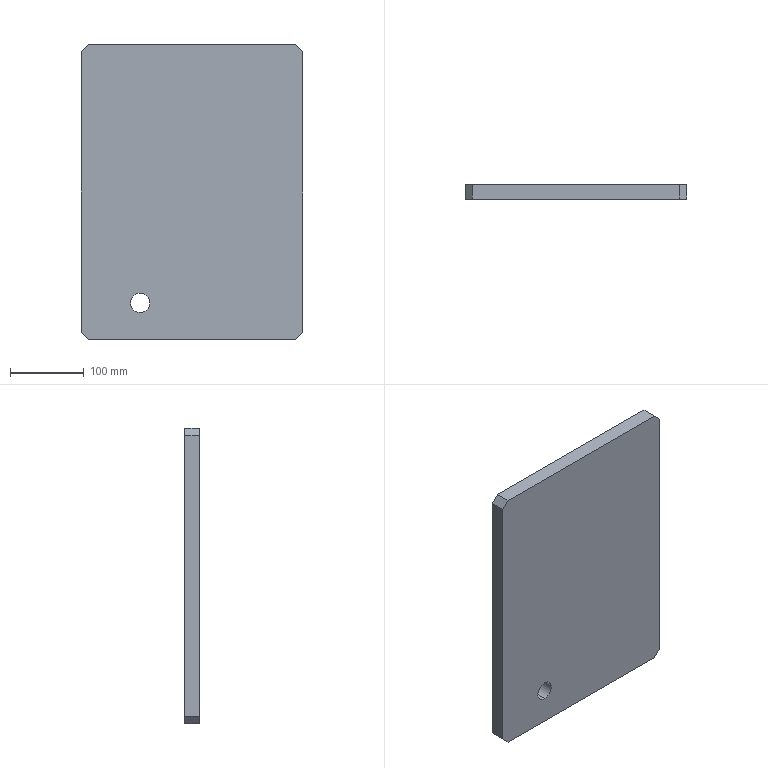Part | SolidWorks | features Chamfer 1, Extrusion 1, HoleWzd 1 | 1 solid | 12 faces | box 300 x 20 x 400 mm | volume 2385381 mm3 | plane 10 | cylinder 2 | commonest cylinder face diameters 26 x2
STEP:
#1=CARTESIAN_POINT('',(-70.,20.,-137.));
#2=VERTEX_POINT('',#1);
#3=CARTESIAN_POINT('',(-70.,20.,-163.));
#4=VERTEX_POINT('',#3);
#5=CARTESIAN_POINT('',(-70.,20.,-150.));
#6=DIRECTION('',(0.,-1.,0.));
#7=DIRECTION('',(0.,0.,-1.));
#8=AXIS2_PLACEMENT_3D('',#5,#6,#7);
#9=CIRCLE('',#8,13.);
#10=EDGE_CURVE('',#2,#4,#9,.T.);
#11=ORIENTED_EDGE('',*,*,#10,.F.);
#12=CARTESIAN_POINT('',(-70.,0.,-137.));
#13=VERTEX_POINT('',#12);
#14=CARTESIAN_POINT('',(-70.,0.,-137.));
#15=DIRECTION('',(0.,-1.,0.));
#16=VECTOR('',#15,1000.);
#17=LINE('',#14,#16);
#18=EDGE_CURVE('',#2,#13,#17,.T.);
#19=ORIENTED_EDGE('',*,*,#18,.T.);
#20=CARTESIAN_POINT('',(-70.,0.,-163.));
#21=VERTEX_POINT('',#20);
#22=CARTESIAN_POINT('',(-70.,0.,-150.));
#23=DIRECTION('',(0.,-1.,0.));
#24=DIRECTION('',(0.,0.,-1.));
#25=AXIS2_PLACEMENT_3D('',#22,#23,#24);
#26=CIRCLE('',#25,13.);
#27=EDGE_CURVE('',#13,#21,#26,.T.);
#28=ORIENTED_EDGE('',*,*,#27,.T.);
#29=CARTESIAN_POINT('',(-70.,0.,-163.));
#30=DIRECTION('',(0.,-1.,0.));
#31=VECTOR('',#30,1000.);
#32=LINE('',#29,#31);
#33=EDGE_CURVE('',#4,#21,#32,.T.);
#34=ORIENTED_EDGE('',*,*,#33,.F.);
#35=EDGE_LOOP('',(#11,#19,#28,#34));
#36=FACE_OUTER_BOUND('',#35,.T.);
#37=CARTESIAN_POINT('',(-70.,0.,-150.));
#38=DIRECTION('',(0.,-1.,0.));
#39=DIRECTION('',(0.,0.,-1.));
#40=AXIS2_PLACEMENT_3D('',#37,#38,#39);
#41=CYLINDRICAL_SURFACE('',#40,13.);
#42=ADVANCED_FACE('',(#36),#41,.F.);
#43=CARTESIAN_POINT('',(150.,20.,190.));
#44=VERTEX_POINT('',#43);
#45=CARTESIAN_POINT('',(150.,20.,-190.));
#46=VERTEX_POINT('',#45);
#47=CARTESIAN_POINT('',(150.,20.,200.));
#48=DIRECTION('',(0.,0.,-1.));
#49=VECTOR('',#48,1000.);
#50=LINE('',#47,#49);
#51=EDGE_CURVE('',#44,#46,#50,.T.);
#52=ORIENTED_EDGE('',*,*,#51,.F.);
#53=CARTESIAN_POINT('',(150.,0.,190.));
#54=VERTEX_POINT('',#53);
#55=CARTESIAN_POINT('',(150.,20.,190.));
#56=DIRECTION('',(0.,-1.,0.));
#57=VECTOR('',#56,1000.);
#58=LINE('',#55,#57);
#59=EDGE_CURVE('',#44,#54,#58,.T.);
#60=ORIENTED_EDGE('',*,*,#59,.T.);
#61=CARTESIAN_POINT('',(150.,0.,-190.));
#62=VERTEX_POINT('',#61);
#63=CARTESIAN_POINT('',(150.,0.,200.));
#64=DIRECTION('',(0.,0.,-1.));
#65=VECTOR('',#64,1000.);
#66=LINE('',#63,#65);
#67=EDGE_CURVE('',#54,#62,#66,.T.);
#68=ORIENTED_EDGE('',*,*,#67,.T.);
#69=CARTESIAN_POINT('',(150.,20.,-190.));
#70=DIRECTION('',(0.,1.,0.));
#71=VECTOR('',#70,1000.);
#72=LINE('',#69,#71);
#73=EDGE_CURVE('',#62,#46,#72,.T.);
#74=ORIENTED_EDGE('',*,*,#73,.T.);
#75=EDGE_LOOP('',(#52,#60,#68,#74));
#76=FACE_OUTER_BOUND('',#75,.T.);
#77=CARTESIAN_POINT('',(150.,20.,200.));
#78=DIRECTION('',(-1.,0.,0.));
#79=DIRECTION('',(0.,0.,1.));
#80=AXIS2_PLACEMENT_3D('',#77,#78,#79);
#81=PLANE('',#80);
#82=ADVANCED_FACE('',(#76),#81,.F.);
#83=CARTESIAN_POINT('',(140.,0.,-200.));
#84=VERTEX_POINT('',#83);
#85=CARTESIAN_POINT('',(-140.,0.,-200.));
#86=VERTEX_POINT('',#85);
#87=CARTESIAN_POINT('',(-150.,0.,-200.));
#88=DIRECTION('',(-1.,0.,0.));
#89=VECTOR('',#88,1000.);
#90=LINE('',#87,#89);
#91=EDGE_CURVE('',#84,#86,#90,.T.);
#92=ORIENTED_EDGE('',*,*,#91,.T.);
#93=CARTESIAN_POINT('',(-140.,20.,-200.));
#94=VERTEX_POINT('',#93);
#95=CARTESIAN_POINT('',(-140.,20.,-200.));
#96=DIRECTION('',(0.,1.,0.));
#97=VECTOR('',#96,1000.);
#98=LINE('',#95,#97);
#99=EDGE_CURVE('',#86,#94,#98,.T.);
#100=ORIENTED_EDGE('',*,*,#99,.T.);
#101=CARTESIAN_POINT('',(140.,20.,-200.));
#102=VERTEX_POINT('',#101);
#103=CARTESIAN_POINT('',(-150.,20.,-200.));
#104=DIRECTION('',(-1.,0.,0.));
#105=VECTOR('',#104,1000.);
#106=LINE('',#103,#105);
#107=EDGE_CURVE('',#102,#94,#106,.T.);
#108=ORIENTED_EDGE('',*,*,#107,.F.);
#109=CARTESIAN_POINT('',(140.,20.,-200.));
#110=DIRECTION('',(0.,-1.,0.));
#111=VECTOR('',#110,1000.);
#112=LINE('',#109,#111);
#113=EDGE_CURVE('',#102,#84,#112,.T.);
#114=ORIENTED_EDGE('',*,*,#113,.T.);
#115=EDGE_LOOP('',(#92,#100,#108,#114));
#116=FACE_OUTER_BOUND('',#115,.T.);
#117=CARTESIAN_POINT('',(-150.,20.,-200.));
#118=DIRECTION('',(0.,0.,1.));
#119=DIRECTION('',(1.,0.,0.));
#120=AXIS2_PLACEMENT_3D('',#117,#118,#119);
#121=PLANE('',#120);
#122=ADVANCED_FACE('',(#116),#121,.F.);
#123=CARTESIAN_POINT('',(-150.,0.,-190.));
#124=VERTEX_POINT('',#123);
#125=CARTESIAN_POINT('',(-150.,0.,190.));
#126=VERTEX_POINT('',#125);
#127=CARTESIAN_POINT('',(-150.,0.,200.));
#128=DIRECTION('',(0.,0.,1.));
#129=VECTOR('',#128,1000.);
#130=LINE('',#127,#129);
#131=EDGE_CURVE('',#124,#126,#130,.T.);
#132=ORIENTED_EDGE('',*,*,#131,.T.);
#133=CARTESIAN_POINT('',(-150.,20.,190.));
#134=VERTEX_POINT('',#133);
#135=CARTESIAN_POINT('',(-150.,20.,190.));
#136=DIRECTION('',(0.,1.,0.));
#137=VECTOR('',#136,1000.);
#138=LINE('',#135,#137);
#139=EDGE_CURVE('',#126,#134,#138,.T.);
#140=ORIENTED_EDGE('',*,*,#139,.T.);
#141=CARTESIAN_POINT('',(-150.,20.,-190.));
#142=VERTEX_POINT('',#141);
#143=CARTESIAN_POINT('',(-150.,20.,200.));
#144=DIRECTION('',(0.,0.,1.));
#145=VECTOR('',#144,1000.);
#146=LINE('',#143,#145);
#147=EDGE_CURVE('',#142,#134,#146,.T.);
#148=ORIENTED_EDGE('',*,*,#147,.F.);
#149=CARTESIAN_POINT('',(-150.,20.,-190.));
#150=DIRECTION('',(0.,-1.,0.));
#151=VECTOR('',#150,1000.);
#152=LINE('',#149,#151);
#153=EDGE_CURVE('',#142,#124,#152,.T.);
#154=ORIENTED_EDGE('',*,*,#153,.T.);
#155=EDGE_LOOP('',(#132,#140,#148,#154));
#156=FACE_OUTER_BOUND('',#155,.T.);
#157=CARTESIAN_POINT('',(-150.,20.,200.));
#158=DIRECTION('',(1.,0.,0.));
#159=DIRECTION('',(0.,0.,-1.));
#160=AXIS2_PLACEMENT_3D('',#157,#158,#159);
#161=PLANE('',#160);
#162=ADVANCED_FACE('',(#156),#161,.F.);
#163=CARTESIAN_POINT('',(-140.,0.,200.));
#164=VERTEX_POINT('',#163);
#165=CARTESIAN_POINT('',(140.,0.,200.));
#166=VERTEX_POINT('',#165);
#167=CARTESIAN_POINT('',(-150.,0.,200.));
#168=DIRECTION('',(1.,0.,0.));
#169=VECTOR('',#168,1000.);
#170=LINE('',#167,#169);
#171=EDGE_CURVE('',#164,#166,#170,.T.);
#172=ORIENTED_EDGE('',*,*,#171,.T.);
#173=CARTESIAN_POINT('',(140.,20.,200.));
#174=VERTEX_POINT('',#173);
#175=CARTESIAN_POINT('',(140.,20.,200.));
#176=DIRECTION('',(0.,1.,0.));
#177=VECTOR('',#176,1000.);
#178=LINE('',#175,#177);
#179=EDGE_CURVE('',#166,#174,#178,.T.);
#180=ORIENTED_EDGE('',*,*,#179,.T.);
#181=CARTESIAN_POINT('',(-140.,20.,200.));
#182=VERTEX_POINT('',#181);
#183=CARTESIAN_POINT('',(-150.,20.,200.));
#184=DIRECTION('',(1.,0.,0.));
#185=VECTOR('',#184,1000.);
#186=LINE('',#183,#185);
#187=EDGE_CURVE('',#182,#174,#186,.T.);
#188=ORIENTED_EDGE('',*,*,#187,.F.);
#189=CARTESIAN_POINT('',(-140.,20.,200.));
#190=DIRECTION('',(0.,-1.,0.));
#191=VECTOR('',#190,1000.);
#192=LINE('',#189,#191);
#193=EDGE_CURVE('',#182,#164,#192,.T.);
#194=ORIENTED_EDGE('',*,*,#193,.T.);
#195=EDGE_LOOP('',(#172,#180,#188,#194));
#196=FACE_OUTER_BOUND('',#195,.T.);
#197=CARTESIAN_POINT('',(-150.,20.,200.));
#198=DIRECTION('',(0.,0.,-1.));
#199=DIRECTION('',(-1.,0.,0.));
#200=AXIS2_PLACEMENT_3D('',#197,#198,#199);
#201=PLANE('',#200);
#202=ADVANCED_FACE('',(#196),#201,.F.);
#203=CARTESIAN_POINT('',(-70.,20.,-150.));
#204=DIRECTION('',(0.,-1.,0.));
#205=DIRECTION('',(0.,0.,-1.));
#206=AXIS2_PLACEMENT_3D('',#203,#204,#205);
#207=CIRCLE('',#206,13.);
#208=EDGE_CURVE('',#4,#2,#207,.T.);
#209=ORIENTED_EDGE('',*,*,#208,.T.);
#210=ORIENTED_EDGE('',*,*,#10,.T.);
#211=EDGE_LOOP('',(#209,#210));
#212=FACE_BOUND('',#211,.T.);
#213=ORIENTED_EDGE('',*,*,#187,.T.);
#214=CARTESIAN_POINT('',(150.,20.,190.));
#215=DIRECTION('',(0.7071,0.,-0.7071));
#216=VECTOR('',#215,1000.);
#217=LINE('',#214,#216);
#218=EDGE_CURVE('',#174,#44,#217,.T.);
#219=ORIENTED_EDGE('',*,*,#218,.T.);
#220=ORIENTED_EDGE('',*,*,#51,.T.);
#221=CARTESIAN_POINT('',(140.,20.,-200.));
#222=DIRECTION('',(-0.7071,0.,-0.7071));
#223=VECTOR('',#222,1000.);
#224=LINE('',#221,#223);
#225=EDGE_CURVE('',#46,#102,#224,.T.);
#226=ORIENTED_EDGE('',*,*,#225,.T.);
#227=ORIENTED_EDGE('',*,*,#107,.T.);
#228=CARTESIAN_POINT('',(-150.,20.,-190.));
#229=DIRECTION('',(-0.7071,0.,0.7071));
#230=VECTOR('',#229,1000.);
#231=LINE('',#228,#230);
#232=EDGE_CURVE('',#94,#142,#231,.T.);
#233=ORIENTED_EDGE('',*,*,#232,.T.);
#234=ORIENTED_EDGE('',*,*,#147,.T.);
#235=CARTESIAN_POINT('',(-140.,20.,200.));
#236=DIRECTION('',(0.7071,0.,0.7071));
#237=VECTOR('',#236,1000.);
#238=LINE('',#235,#237);
#239=EDGE_CURVE('',#134,#182,#238,.T.);
#240=ORIENTED_EDGE('',*,*,#239,.T.);
#241=EDGE_LOOP('',(#213,#219,#220,#226,#227,#233,#234,#240));
#242=FACE_OUTER_BOUND('',#241,.T.);
#243=CARTESIAN_POINT('',(0.,20.,0.));
#244=DIRECTION('',(0.,-1.,0.));
#245=DIRECTION('',(0.,0.,-1.));
#246=AXIS2_PLACEMENT_3D('',#243,#244,#245);
#247=PLANE('',#246);
#248=ADVANCED_FACE('',(#212,#242),#247,.F.);
#249=CARTESIAN_POINT('',(-70.,0.,-150.));
#250=DIRECTION('',(0.,-1.,0.));
#251=DIRECTION('',(0.,0.,-1.));
#252=AXIS2_PLACEMENT_3D('',#249,#250,#251);
#253=CIRCLE('',#252,13.);
#254=EDGE_CURVE('',#21,#13,#253,.T.);
#255=ORIENTED_EDGE('',*,*,#254,.F.);
#256=ORIENTED_EDGE('',*,*,#27,.F.);
#257=EDGE_LOOP('',(#255,#256));
#258=FACE_BOUND('',#257,.T.);
#259=ORIENTED_EDGE('',*,*,#67,.F.);
#260=CARTESIAN_POINT('',(170.,0.,170.));
#261=DIRECTION('',(-0.7071,0.,0.7071));
#262=VECTOR('',#261,1000.);
#263=LINE('',#260,#262);
#264=EDGE_CURVE('',#54,#166,#263,.T.);
#265=ORIENTED_EDGE('',*,*,#264,.T.);
#266=ORIENTED_EDGE('',*,*,#171,.F.);
#267=CARTESIAN_POINT('',(-170.,0.,170.));
#268=DIRECTION('',(-0.7071,0.,-0.7071));
#269=VECTOR('',#268,1000.);
#270=LINE('',#267,#269);
#271=EDGE_CURVE('',#164,#126,#270,.T.);
#272=ORIENTED_EDGE('',*,*,#271,.T.);
#273=ORIENTED_EDGE('',*,*,#131,.F.);
#274=CARTESIAN_POINT('',(-170.,0.,-170.));
#275=DIRECTION('',(0.7071,0.,-0.7071));
#276=VECTOR('',#275,1000.);
#277=LINE('',#274,#276);
#278=EDGE_CURVE('',#124,#86,#277,.T.);
#279=ORIENTED_EDGE('',*,*,#278,.T.);
#280=ORIENTED_EDGE('',*,*,#91,.F.);
#281=CARTESIAN_POINT('',(170.,0.,-170.));
#282=DIRECTION('',(0.7071,0.,0.7071));
#283=VECTOR('',#282,1000.);
#284=LINE('',#281,#283);
#285=EDGE_CURVE('',#84,#62,#284,.T.);
#286=ORIENTED_EDGE('',*,*,#285,.T.);
#287=EDGE_LOOP('',(#259,#265,#266,#272,#273,#279,#280,#286));
#288=FACE_OUTER_BOUND('',#287,.T.);
#289=CARTESIAN_POINT('',(0.,0.,0.));
#290=DIRECTION('',(0.,-1.,0.));
#291=DIRECTION('',(0.,0.,-1.));
#292=AXIS2_PLACEMENT_3D('',#289,#290,#291);
#293=PLANE('',#292);
#294=ADVANCED_FACE('',(#258,#288),#293,.T.);
#295=ORIENTED_EDGE('',*,*,#218,.F.);
#296=ORIENTED_EDGE('',*,*,#179,.F.);
#297=ORIENTED_EDGE('',*,*,#264,.F.);
#298=ORIENTED_EDGE('',*,*,#59,.F.);
#299=EDGE_LOOP('',(#295,#296,#297,#298));
#300=FACE_OUTER_BOUND('',#299,.T.);
#301=CARTESIAN_POINT('',(150.,20.,190.));
#302=DIRECTION('',(-0.7071,0.,-0.7071));
#303=DIRECTION('',(0.,-1.,0.));
#304=AXIS2_PLACEMENT_3D('',#301,#302,#303);
#305=PLANE('',#304);
#306=ADVANCED_FACE('',(#300),#305,.F.);
#307=ORIENTED_EDGE('',*,*,#239,.F.);
#308=ORIENTED_EDGE('',*,*,#139,.F.);
#309=ORIENTED_EDGE('',*,*,#271,.F.);
#310=ORIENTED_EDGE('',*,*,#193,.F.);
#311=EDGE_LOOP('',(#307,#308,#309,#310));
#312=FACE_OUTER_BOUND('',#311,.T.);
#313=CARTESIAN_POINT('',(-140.,20.,200.));
#314=DIRECTION('',(0.7071,0.,-0.7071));
#315=DIRECTION('',(0.,-1.,0.));
#316=AXIS2_PLACEMENT_3D('',#313,#314,#315);
#317=PLANE('',#316);
#318=ADVANCED_FACE('',(#312),#317,.F.);
#319=ORIENTED_EDGE('',*,*,#232,.F.);
#320=ORIENTED_EDGE('',*,*,#99,.F.);
#321=ORIENTED_EDGE('',*,*,#278,.F.);
#322=ORIENTED_EDGE('',*,*,#153,.F.);
#323=EDGE_LOOP('',(#319,#320,#321,#322));
#324=FACE_OUTER_BOUND('',#323,.T.);
#325=CARTESIAN_POINT('',(-150.,20.,-190.));
#326=DIRECTION('',(0.7071,0.,0.7071));
#327=DIRECTION('',(0.,-1.,0.));
#328=AXIS2_PLACEMENT_3D('',#325,#326,#327);
#329=PLANE('',#328);
#330=ADVANCED_FACE('',(#324),#329,.F.);
#331=ORIENTED_EDGE('',*,*,#225,.F.);
#332=ORIENTED_EDGE('',*,*,#73,.F.);
#333=ORIENTED_EDGE('',*,*,#285,.F.);
#334=ORIENTED_EDGE('',*,*,#113,.F.);
#335=EDGE_LOOP('',(#331,#332,#333,#334));
#336=FACE_OUTER_BOUND('',#335,.T.);
#337=CARTESIAN_POINT('',(140.,20.,-200.));
#338=DIRECTION('',(-0.7071,0.,0.7071));
#339=DIRECTION('',(0.,-1.,0.));
#340=AXIS2_PLACEMENT_3D('',#337,#338,#339);
#341=PLANE('',#340);
#342=ADVANCED_FACE('',(#336),#341,.F.);
#343=ORIENTED_EDGE('',*,*,#18,.F.);
#344=ORIENTED_EDGE('',*,*,#208,.F.);
#345=ORIENTED_EDGE('',*,*,#33,.T.);
#346=ORIENTED_EDGE('',*,*,#254,.T.);
#347=EDGE_LOOP('',(#343,#344,#345,#346));
#348=FACE_OUTER_BOUND('',#347,.T.);
#349=CARTESIAN_POINT('',(-70.,0.,-150.));
#350=DIRECTION('',(0.,-1.,0.));
#351=DIRECTION('',(0.,0.,-1.));
#352=AXIS2_PLACEMENT_3D('',#349,#350,#351);
#353=CYLINDRICAL_SURFACE('',#352,13.);
#354=ADVANCED_FACE('',(#348),#353,.F.);
#355=CLOSED_SHELL('',(#42,#82,#122,#162,#202,#248,#294,#306,#318,#330,#342,#354));
#356=MANIFOLD_SOLID_BREP('',#355);
#357=CARTESIAN_POINT('',(0.,0.,0.));
#358=DIRECTION('',(0.,0.,1.));
#359=DIRECTION('',(1.,0.,0.));
#360=AXIS2_PLACEMENT_3D('',#357,#358,#359);
#361=(LENGTH_UNIT()NAMED_UNIT(*)SI_UNIT(.MILLI.,.METRE.));
#362=UNCERTAINTY_MEASURE_WITH_UNIT(LENGTH_MEASURE(0.00001),#361,'','');
#363=(NAMED_UNIT(*)PLANE_ANGLE_UNIT()SI_UNIT($,.RADIAN.));
#364=(NAMED_UNIT(*)SI_UNIT($,.STERADIAN.)SOLID_ANGLE_UNIT());
#365=(GEOMETRIC_REPRESENTATION_CONTEXT(3)GLOBAL_UNCERTAINTY_ASSIGNED_CONTEXT((#362))GLOBAL_UNIT_ASSIGNED_CONTEXT((#361,#363,#364))REPRESENTATION_CONTEXT('',''));
#366=ADVANCED_BREP_SHAPE_REPRESENTATION('',(#356,#360),#365);